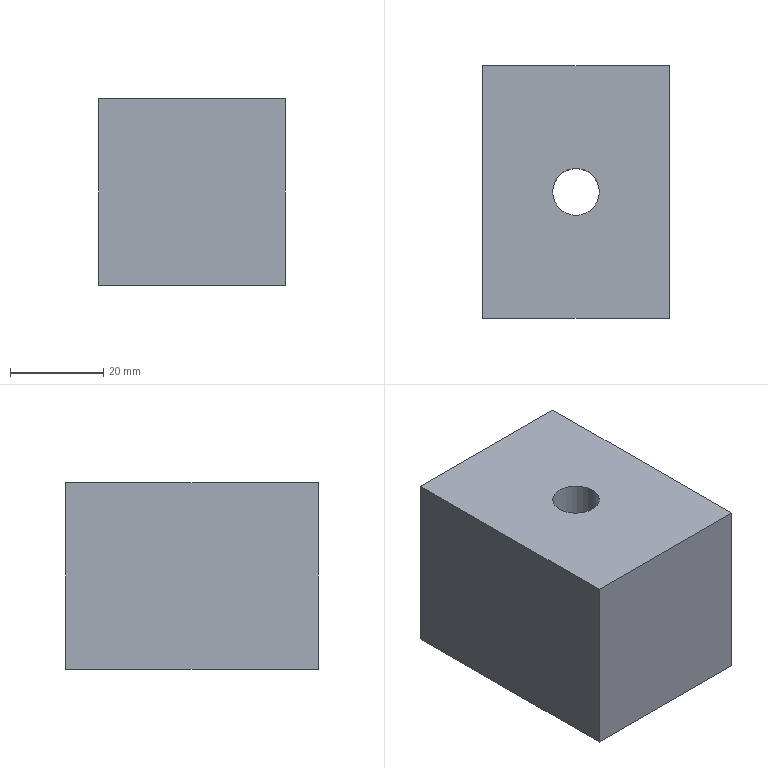Part | STEP file | 1 solid | 8 faces | box 40 x 54 x 40 mm | volume 83258 mm3 | plane 6 | cylinder 2 | commonest cylinder face diameters 10 x2
STEP:
#1=CARTESIAN_POINT('',(0.,0.,0.));
#2=DIRECTION('',(0.,0.,1.));
#3=DIRECTION('',(1.,0.,0.));
#4=AXIS2_PLACEMENT_3D('',#1,#2,#3);
#5=CARTESIAN_POINT('',(5.,0.,0.));
#6=VERTEX_POINT('',#5);
#7=CARTESIAN_POINT('',(5.,0.,40.));
#8=VERTEX_POINT('',#7);
#9=CARTESIAN_POINT('',(5.,0.,40.));
#10=DIRECTION('',(0.,0.,1.));
#11=VECTOR('',#10,1.);
#12=LINE('',#9,#11);
#13=CARTESIAN_POINT('',(0.,0.,40.));
#14=DIRECTION('',(0.,0.,1.));
#15=DIRECTION('',(1.,0.,0.));
#16=AXIS2_PLACEMENT_3D('',#13,#14,#15);
#17=CYLINDRICAL_SURFACE('',#16,5.);
#18=CARTESIAN_POINT('',(6.283,0.));
#19=DIRECTION('',(0.,1.));
#20=VECTOR('',#19,1.);
#21=LINE('',#18,#20);
#22=(GEOMETRIC_REPRESENTATION_CONTEXT(2)PARAMETRIC_REPRESENTATION_CONTEXT()REPRESENTATION_CONTEXT('',''));
#23=DEFINITIONAL_REPRESENTATION('',(#21),#22);
#24=PCURVE('',#17,#23);
#25=CARTESIAN_POINT('',(0.,0.,40.));
#26=DIRECTION('',(0.,0.,1.));
#27=DIRECTION('',(1.,0.,0.));
#28=AXIS2_PLACEMENT_3D('',#25,#26,#27);
#29=CYLINDRICAL_SURFACE('',#28,5.);
#30=CARTESIAN_POINT('',(0.,0.));
#31=DIRECTION('',(0.,1.));
#32=VECTOR('',#31,1.);
#33=LINE('',#30,#32);
#34=(GEOMETRIC_REPRESENTATION_CONTEXT(2)PARAMETRIC_REPRESENTATION_CONTEXT()REPRESENTATION_CONTEXT('',''));
#35=DEFINITIONAL_REPRESENTATION('',(#33),#34);
#36=PCURVE('',#29,#35);
#37=SURFACE_CURVE('',#12,(#24,#36),.PCURVE_S1.);
#38=EDGE_CURVE('',#6,#8,#37,.T.);
#39=ORIENTED_EDGE('',*,*,#38,.T.);
#40=CARTESIAN_POINT('',(-5.,0.,40.));
#41=VERTEX_POINT('',#40);
#42=CARTESIAN_POINT('',(0.,0.,40.));
#43=DIRECTION('',(0.,0.,-1.));
#44=DIRECTION('',(1.,0.,0.));
#45=AXIS2_PLACEMENT_3D('',#42,#43,#44);
#46=CIRCLE('',#45,5.);
#47=CARTESIAN_POINT('',(6.283,0.));
#48=DIRECTION('',(-1.,0.));
#49=VECTOR('',#48,1.);
#50=LINE('',#47,#49);
#51=(GEOMETRIC_REPRESENTATION_CONTEXT(2)PARAMETRIC_REPRESENTATION_CONTEXT()REPRESENTATION_CONTEXT('',''));
#52=DEFINITIONAL_REPRESENTATION('',(#50),#51);
#53=PCURVE('',#17,#52);
#54=CARTESIAN_POINT('',(0.,0.,40.));
#55=DIRECTION('',(0.,0.,1.));
#56=DIRECTION('',(1.,0.,0.));
#57=AXIS2_PLACEMENT_3D('',#54,#55,#56);
#58=PLANE('',#57);
#59=CARTESIAN_POINT('',(5.,0.));
#60=CARTESIAN_POINT('',(5.,-8.66));
#61=CARTESIAN_POINT('',(-2.5,-4.33));
#62=CARTESIAN_POINT('',(-10.,0.));
#63=CARTESIAN_POINT('',(-2.5,4.33));
#64=CARTESIAN_POINT('',(5.,8.66));
#65=CARTESIAN_POINT('',(5.,0.));
#66=(BOUNDED_CURVE()B_SPLINE_CURVE(2,(#59,#60,#61,#62,#63,#64,#65),.UNSPECIFIED.,.T.,.F.)B_SPLINE_CURVE_WITH_KNOTS((1,2,2,2,2,1),(-2.094,0.,2.094,4.189,6.283,8.378),.UNSPECIFIED.)CURVE()GEOMETRIC_REPRESENTATION_ITEM()RATIONAL_B_SPLINE_CURVE((1.,0.5,1.,0.5,1.,0.5,1.))REPRESENTATION_ITEM(''));
#67=(GEOMETRIC_REPRESENTATION_CONTEXT(2)PARAMETRIC_REPRESENTATION_CONTEXT()REPRESENTATION_CONTEXT('',''));
#68=DEFINITIONAL_REPRESENTATION('',(#66),#67);
#69=PCURVE('',#58,#68);
#70=SURFACE_CURVE('',#46,(#53,#69),.PCURVE_S1.);
#71=EDGE_CURVE('',#8,#41,#70,.T.);
#72=ORIENTED_EDGE('',*,*,#71,.T.);
#73=CARTESIAN_POINT('',(-5.,0.,0.));
#74=VERTEX_POINT('',#73);
#75=CARTESIAN_POINT('',(-5.,0.,40.));
#76=DIRECTION('',(0.,0.,1.));
#77=VECTOR('',#76,1.);
#78=LINE('',#75,#77);
#79=CARTESIAN_POINT('',(3.142,0.));
#80=DIRECTION('',(0.,1.));
#81=VECTOR('',#80,1.);
#82=LINE('',#79,#81);
#83=(GEOMETRIC_REPRESENTATION_CONTEXT(2)PARAMETRIC_REPRESENTATION_CONTEXT()REPRESENTATION_CONTEXT('',''));
#84=DEFINITIONAL_REPRESENTATION('',(#82),#83);
#85=PCURVE('',#17,#84);
#86=CARTESIAN_POINT('',(3.142,0.));
#87=DIRECTION('',(0.,1.));
#88=VECTOR('',#87,1.);
#89=LINE('',#86,#88);
#90=(GEOMETRIC_REPRESENTATION_CONTEXT(2)PARAMETRIC_REPRESENTATION_CONTEXT()REPRESENTATION_CONTEXT('',''));
#91=DEFINITIONAL_REPRESENTATION('',(#89),#90);
#92=PCURVE('',#29,#91);
#93=SURFACE_CURVE('',#78,(#85,#92),.PCURVE_S1.);
#94=EDGE_CURVE('',#74,#41,#93,.T.);
#95=ORIENTED_EDGE('',*,*,#94,.F.);
#96=CARTESIAN_POINT('',(0.,0.,0.));
#97=DIRECTION('',(0.,0.,-1.));
#98=DIRECTION('',(1.,0.,0.));
#99=AXIS2_PLACEMENT_3D('',#96,#97,#98);
#100=CIRCLE('',#99,5.);
#101=CARTESIAN_POINT('',(6.283,-40.));
#102=DIRECTION('',(-1.,0.));
#103=VECTOR('',#102,1.);
#104=LINE('',#101,#103);
#105=(GEOMETRIC_REPRESENTATION_CONTEXT(2)PARAMETRIC_REPRESENTATION_CONTEXT()REPRESENTATION_CONTEXT('',''));
#106=DEFINITIONAL_REPRESENTATION('',(#104),#105);
#107=PCURVE('',#17,#106);
#108=CARTESIAN_POINT('',(0.,0.,0.));
#109=DIRECTION('',(0.,0.,1.));
#110=DIRECTION('',(1.,0.,0.));
#111=AXIS2_PLACEMENT_3D('',#108,#109,#110);
#112=PLANE('',#111);
#113=CARTESIAN_POINT('',(5.,0.));
#114=CARTESIAN_POINT('',(5.,-8.66));
#115=CARTESIAN_POINT('',(-2.5,-4.33));
#116=CARTESIAN_POINT('',(-10.,0.));
#117=CARTESIAN_POINT('',(-2.5,4.33));
#118=CARTESIAN_POINT('',(5.,8.66));
#119=CARTESIAN_POINT('',(5.,0.));
#120=(BOUNDED_CURVE()B_SPLINE_CURVE(2,(#113,#114,#115,#116,#117,#118,#119),.UNSPECIFIED.,.T.,.F.)B_SPLINE_CURVE_WITH_KNOTS((1,2,2,2,2,1),(-2.094,0.,2.094,4.189,6.283,8.378),.UNSPECIFIED.)CURVE()GEOMETRIC_REPRESENTATION_ITEM()RATIONAL_B_SPLINE_CURVE((1.,0.5,1.,0.5,1.,0.5,1.))REPRESENTATION_ITEM(''));
#121=(GEOMETRIC_REPRESENTATION_CONTEXT(2)PARAMETRIC_REPRESENTATION_CONTEXT()REPRESENTATION_CONTEXT('',''));
#122=DEFINITIONAL_REPRESENTATION('',(#120),#121);
#123=PCURVE('',#112,#122);
#124=SURFACE_CURVE('',#100,(#107,#123),.PCURVE_S1.);
#125=EDGE_CURVE('',#6,#74,#124,.T.);
#126=ORIENTED_EDGE('',*,*,#125,.F.);
#127=EDGE_LOOP('',(#39,#72,#95,#126));
#128=FACE_BOUND('',#127,.F.);
#129=ADVANCED_FACE('',(#128),#17,.F.);
#130=CARTESIAN_POINT('',(20.,27.,40.));
#131=VERTEX_POINT('',#130);
#132=CARTESIAN_POINT('',(20.,27.,0.));
#133=VERTEX_POINT('',#132);
#134=CARTESIAN_POINT('',(20.,27.,40.));
#135=DIRECTION('',(0.,0.,-1.));
#136=VECTOR('',#135,1.);
#137=LINE('',#134,#136);
#138=CARTESIAN_POINT('',(20.,27.,40.));
#139=DIRECTION('',(-1.,0.,0.));
#140=DIRECTION('',(0.,-1.,0.));
#141=AXIS2_PLACEMENT_3D('',#138,#139,#140);
#142=PLANE('',#141);
#143=CARTESIAN_POINT('',(0.,0.));
#144=DIRECTION('',(0.,-1.));
#145=VECTOR('',#144,1.);
#146=LINE('',#143,#145);
#147=(GEOMETRIC_REPRESENTATION_CONTEXT(2)PARAMETRIC_REPRESENTATION_CONTEXT()REPRESENTATION_CONTEXT('',''));
#148=DEFINITIONAL_REPRESENTATION('',(#146),#147);
#149=PCURVE('',#142,#148);
#150=CARTESIAN_POINT('',(-20.,27.,40.));
#151=DIRECTION('',(0.,-1.,0.));
#152=DIRECTION('',(0.,0.,-1.));
#153=AXIS2_PLACEMENT_3D('',#150,#151,#152);
#154=PLANE('',#153);
#155=CARTESIAN_POINT('',(0.,40.));
#156=DIRECTION('',(1.,0.));
#157=VECTOR('',#156,1.);
#158=LINE('',#155,#157);
#159=(GEOMETRIC_REPRESENTATION_CONTEXT(2)PARAMETRIC_REPRESENTATION_CONTEXT()REPRESENTATION_CONTEXT('',''));
#160=DEFINITIONAL_REPRESENTATION('',(#158),#159);
#161=PCURVE('',#154,#160);
#162=SURFACE_CURVE('',#137,(#149,#161),.PCURVE_S1.);
#163=EDGE_CURVE('',#131,#133,#162,.T.);
#164=ORIENTED_EDGE('',*,*,#163,.F.);
#165=CARTESIAN_POINT('',(20.,-27.,40.));
#166=VERTEX_POINT('',#165);
#167=CARTESIAN_POINT('',(20.,27.,40.));
#168=DIRECTION('',(0.,1.,0.));
#169=VECTOR('',#168,1.);
#170=LINE('',#167,#169);
#171=CARTESIAN_POINT('',(0.,0.));
#172=DIRECTION('',(-1.,0.));
#173=VECTOR('',#172,1.);
#174=LINE('',#171,#173);
#175=(GEOMETRIC_REPRESENTATION_CONTEXT(2)PARAMETRIC_REPRESENTATION_CONTEXT()REPRESENTATION_CONTEXT('',''));
#176=DEFINITIONAL_REPRESENTATION('',(#174),#175);
#177=PCURVE('',#142,#176);
#178=CARTESIAN_POINT('',(20.,27.));
#179=DIRECTION('',(0.,1.));
#180=VECTOR('',#179,1.);
#181=LINE('',#178,#180);
#182=(GEOMETRIC_REPRESENTATION_CONTEXT(2)PARAMETRIC_REPRESENTATION_CONTEXT()REPRESENTATION_CONTEXT('',''));
#183=DEFINITIONAL_REPRESENTATION('',(#181),#182);
#184=PCURVE('',#58,#183);
#185=SURFACE_CURVE('',#170,(#177,#184),.PCURVE_S1.);
#186=EDGE_CURVE('',#166,#131,#185,.T.);
#187=ORIENTED_EDGE('',*,*,#186,.F.);
#188=CARTESIAN_POINT('',(20.,-27.,0.));
#189=VERTEX_POINT('',#188);
#190=CARTESIAN_POINT('',(20.,-27.,40.));
#191=DIRECTION('',(0.,0.,1.));
#192=VECTOR('',#191,1.);
#193=LINE('',#190,#192);
#194=CARTESIAN_POINT('',(54.,0.));
#195=DIRECTION('',(0.,1.));
#196=VECTOR('',#195,1.);
#197=LINE('',#194,#196);
#198=(GEOMETRIC_REPRESENTATION_CONTEXT(2)PARAMETRIC_REPRESENTATION_CONTEXT()REPRESENTATION_CONTEXT('',''));
#199=DEFINITIONAL_REPRESENTATION('',(#197),#198);
#200=PCURVE('',#142,#199);
#201=CARTESIAN_POINT('',(-20.,-27.,40.));
#202=DIRECTION('',(0.,1.,0.));
#203=DIRECTION('',(0.,0.,1.));
#204=AXIS2_PLACEMENT_3D('',#201,#202,#203);
#205=PLANE('',#204);
#206=CARTESIAN_POINT('',(0.,40.));
#207=DIRECTION('',(1.,0.));
#208=VECTOR('',#207,1.);
#209=LINE('',#206,#208);
#210=(GEOMETRIC_REPRESENTATION_CONTEXT(2)PARAMETRIC_REPRESENTATION_CONTEXT()REPRESENTATION_CONTEXT('',''));
#211=DEFINITIONAL_REPRESENTATION('',(#209),#210);
#212=PCURVE('',#205,#211);
#213=SURFACE_CURVE('',#193,(#200,#212),.PCURVE_S1.);
#214=EDGE_CURVE('',#189,#166,#213,.T.);
#215=ORIENTED_EDGE('',*,*,#214,.F.);
#216=CARTESIAN_POINT('',(20.,27.,0.));
#217=DIRECTION('',(0.,-1.,0.));
#218=VECTOR('',#217,1.);
#219=LINE('',#216,#218);
#220=CARTESIAN_POINT('',(0.,-40.));
#221=DIRECTION('',(1.,0.));
#222=VECTOR('',#221,1.);
#223=LINE('',#220,#222);
#224=(GEOMETRIC_REPRESENTATION_CONTEXT(2)PARAMETRIC_REPRESENTATION_CONTEXT()REPRESENTATION_CONTEXT('',''));
#225=DEFINITIONAL_REPRESENTATION('',(#223),#224);
#226=PCURVE('',#142,#225);
#227=CARTESIAN_POINT('',(20.,27.));
#228=DIRECTION('',(0.,-1.));
#229=VECTOR('',#228,1.);
#230=LINE('',#227,#229);
#231=(GEOMETRIC_REPRESENTATION_CONTEXT(2)PARAMETRIC_REPRESENTATION_CONTEXT()REPRESENTATION_CONTEXT('',''));
#232=DEFINITIONAL_REPRESENTATION('',(#230),#231);
#233=PCURVE('',#112,#232);
#234=SURFACE_CURVE('',#219,(#226,#233),.PCURVE_S1.);
#235=EDGE_CURVE('',#133,#189,#234,.T.);
#236=ORIENTED_EDGE('',*,*,#235,.F.);
#237=EDGE_LOOP('',(#164,#187,#215,#236));
#238=FACE_BOUND('',#237,.T.);
#239=ADVANCED_FACE('',(#238),#142,.F.);
#240=ORIENTED_EDGE('',*,*,#125,.F.);
#241=CARTESIAN_POINT('',(0.,0.,0.));
#242=DIRECTION('',(0.,0.,-1.));
#243=DIRECTION('',(1.,0.,0.));
#244=AXIS2_PLACEMENT_3D('',#241,#242,#243);
#245=CIRCLE('',#244,5.);
#246=CARTESIAN_POINT('',(5.,0.));
#247=CARTESIAN_POINT('',(5.,-8.66));
#248=CARTESIAN_POINT('',(-2.5,-4.33));
#249=CARTESIAN_POINT('',(-10.,0.));
#250=CARTESIAN_POINT('',(-2.5,4.33));
#251=CARTESIAN_POINT('',(5.,8.66));
#252=CARTESIAN_POINT('',(5.,0.));
#253=(BOUNDED_CURVE()B_SPLINE_CURVE(2,(#246,#247,#248,#249,#250,#251,#252),.UNSPECIFIED.,.T.,.F.)B_SPLINE_CURVE_WITH_KNOTS((1,2,2,2,2,1),(-2.094,0.,2.094,4.189,6.283,8.378),.UNSPECIFIED.)CURVE()GEOMETRIC_REPRESENTATION_ITEM()RATIONAL_B_SPLINE_CURVE((1.,0.5,1.,0.5,1.,0.5,1.))REPRESENTATION_ITEM(''));
#254=(GEOMETRIC_REPRESENTATION_CONTEXT(2)PARAMETRIC_REPRESENTATION_CONTEXT()REPRESENTATION_CONTEXT('',''));
#255=DEFINITIONAL_REPRESENTATION('',(#253),#254);
#256=PCURVE('',#112,#255);
#257=CARTESIAN_POINT('',(6.283,-40.));
#258=DIRECTION('',(-1.,0.));
#259=VECTOR('',#258,1.);
#260=LINE('',#257,#259);
#261=(GEOMETRIC_REPRESENTATION_CONTEXT(2)PARAMETRIC_REPRESENTATION_CONTEXT()REPRESENTATION_CONTEXT('',''));
#262=DEFINITIONAL_REPRESENTATION('',(#260),#261);
#263=PCURVE('',#29,#262);
#264=SURFACE_CURVE('',#245,(#256,#263),.PCURVE_S1.);
#265=EDGE_CURVE('',#74,#6,#264,.T.);
#266=ORIENTED_EDGE('',*,*,#265,.F.);
#267=EDGE_LOOP('',(#240,#266));
#268=FACE_BOUND('',#267,.T.);
#269=CARTESIAN_POINT('',(-20.,-27.,0.));
#270=VERTEX_POINT('',#269);
#271=CARTESIAN_POINT('',(0.,-27.,0.));
#272=DIRECTION('',(1.,0.,0.));
#273=VECTOR('',#272,1.);
#274=LINE('',#271,#273);
#275=CARTESIAN_POINT('',(0.,-27.));
#276=DIRECTION('',(1.,0.));
#277=VECTOR('',#276,1.);
#278=LINE('',#275,#277);
#279=(GEOMETRIC_REPRESENTATION_CONTEXT(2)PARAMETRIC_REPRESENTATION_CONTEXT()REPRESENTATION_CONTEXT('',''));
#280=DEFINITIONAL_REPRESENTATION('',(#278),#279);
#281=PCURVE('',#112,#280);
#282=CARTESIAN_POINT('',(-40.,20.));
#283=DIRECTION('',(0.,1.));
#284=VECTOR('',#283,1.);
#285=LINE('',#282,#284);
#286=(GEOMETRIC_REPRESENTATION_CONTEXT(2)PARAMETRIC_REPRESENTATION_CONTEXT()REPRESENTATION_CONTEXT('',''));
#287=DEFINITIONAL_REPRESENTATION('',(#285),#286);
#288=PCURVE('',#205,#287);
#289=SURFACE_CURVE('',#274,(#281,#288),.PCURVE_S1.);
#290=EDGE_CURVE('',#270,#189,#289,.T.);
#291=ORIENTED_EDGE('',*,*,#290,.F.);
#292=CARTESIAN_POINT('',(-20.,27.,0.));
#293=VERTEX_POINT('',#292);
#294=CARTESIAN_POINT('',(-20.,0.,0.));
#295=DIRECTION('',(0.,-1.,0.));
#296=VECTOR('',#295,1.);
#297=LINE('',#294,#296);
#298=CARTESIAN_POINT('',(-20.,0.));
#299=DIRECTION('',(0.,-1.));
#300=VECTOR('',#299,1.);
#301=LINE('',#298,#300);
#302=(GEOMETRIC_REPRESENTATION_CONTEXT(2)PARAMETRIC_REPRESENTATION_CONTEXT()REPRESENTATION_CONTEXT('',''));
#303=DEFINITIONAL_REPRESENTATION('',(#301),#302);
#304=PCURVE('',#112,#303);
#305=CARTESIAN_POINT('',(-20.,27.,40.));
#306=DIRECTION('',(1.,0.,0.));
#307=DIRECTION('',(0.,1.,0.));
#308=AXIS2_PLACEMENT_3D('',#305,#306,#307);
#309=PLANE('',#308);
#310=CARTESIAN_POINT('',(-27.,-40.));
#311=DIRECTION('',(-1.,0.));
#312=VECTOR('',#311,1.);
#313=LINE('',#310,#312);
#314=(GEOMETRIC_REPRESENTATION_CONTEXT(2)PARAMETRIC_REPRESENTATION_CONTEXT()REPRESENTATION_CONTEXT('',''));
#315=DEFINITIONAL_REPRESENTATION('',(#313),#314);
#316=PCURVE('',#309,#315);
#317=SURFACE_CURVE('',#297,(#304,#316),.PCURVE_S1.);
#318=EDGE_CURVE('',#293,#270,#317,.T.);
#319=ORIENTED_EDGE('',*,*,#318,.F.);
#320=CARTESIAN_POINT('',(0.,27.,0.));
#321=DIRECTION('',(-1.,0.,0.));
#322=VECTOR('',#321,1.);
#323=LINE('',#320,#322);
#324=CARTESIAN_POINT('',(0.,27.));
#325=DIRECTION('',(-1.,0.));
#326=VECTOR('',#325,1.);
#327=LINE('',#324,#326);
#328=(GEOMETRIC_REPRESENTATION_CONTEXT(2)PARAMETRIC_REPRESENTATION_CONTEXT()REPRESENTATION_CONTEXT('',''));
#329=DEFINITIONAL_REPRESENTATION('',(#327),#328);
#330=PCURVE('',#112,#329);
#331=CARTESIAN_POINT('',(40.,20.));
#332=DIRECTION('',(0.,-1.));
#333=VECTOR('',#332,1.);
#334=LINE('',#331,#333);
#335=(GEOMETRIC_REPRESENTATION_CONTEXT(2)PARAMETRIC_REPRESENTATION_CONTEXT()REPRESENTATION_CONTEXT('',''));
#336=DEFINITIONAL_REPRESENTATION('',(#334),#335);
#337=PCURVE('',#154,#336);
#338=SURFACE_CURVE('',#323,(#330,#337),.PCURVE_S1.);
#339=EDGE_CURVE('',#133,#293,#338,.T.);
#340=ORIENTED_EDGE('',*,*,#339,.F.);
#341=ORIENTED_EDGE('',*,*,#235,.T.);
#342=EDGE_LOOP('',(#291,#319,#340,#341));
#343=FACE_BOUND('',#342,.T.);
#344=ADVANCED_FACE('',(#268,#343),#112,.F.);
#345=CARTESIAN_POINT('',(-20.,27.,40.));
#346=VERTEX_POINT('',#345);
#347=CARTESIAN_POINT('',(-20.,27.,40.));
#348=DIRECTION('',(0.,0.,-1.));
#349=VECTOR('',#348,1.);
#350=LINE('',#347,#349);
#351=CARTESIAN_POINT('',(0.,0.));
#352=DIRECTION('',(1.,0.));
#353=VECTOR('',#352,1.);
#354=LINE('',#351,#353);
#355=(GEOMETRIC_REPRESENTATION_CONTEXT(2)PARAMETRIC_REPRESENTATION_CONTEXT()REPRESENTATION_CONTEXT('',''));
#356=DEFINITIONAL_REPRESENTATION('',(#354),#355);
#357=PCURVE('',#154,#356);
#358=CARTESIAN_POINT('',(0.,0.));
#359=DIRECTION('',(0.,-1.));
#360=VECTOR('',#359,1.);
#361=LINE('',#358,#360);
#362=(GEOMETRIC_REPRESENTATION_CONTEXT(2)PARAMETRIC_REPRESENTATION_CONTEXT()REPRESENTATION_CONTEXT('',''));
#363=DEFINITIONAL_REPRESENTATION('',(#361),#362);
#364=PCURVE('',#309,#363);
#365=SURFACE_CURVE('',#350,(#357,#364),.PCURVE_S1.);
#366=EDGE_CURVE('',#346,#293,#365,.T.);
#367=ORIENTED_EDGE('',*,*,#366,.F.);
#368=CARTESIAN_POINT('',(-20.,27.,40.));
#369=DIRECTION('',(-1.,0.,0.));
#370=VECTOR('',#369,1.);
#371=LINE('',#368,#370);
#372=CARTESIAN_POINT('',(0.,0.));
#373=DIRECTION('',(0.,-1.));
#374=VECTOR('',#373,1.);
#375=LINE('',#372,#374);
#376=(GEOMETRIC_REPRESENTATION_CONTEXT(2)PARAMETRIC_REPRESENTATION_CONTEXT()REPRESENTATION_CONTEXT('',''));
#377=DEFINITIONAL_REPRESENTATION('',(#375),#376);
#378=PCURVE('',#154,#377);
#379=CARTESIAN_POINT('',(-20.,27.));
#380=DIRECTION('',(-1.,0.));
#381=VECTOR('',#380,1.);
#382=LINE('',#379,#381);
#383=(GEOMETRIC_REPRESENTATION_CONTEXT(2)PARAMETRIC_REPRESENTATION_CONTEXT()REPRESENTATION_CONTEXT('',''));
#384=DEFINITIONAL_REPRESENTATION('',(#382),#383);
#385=PCURVE('',#58,#384);
#386=SURFACE_CURVE('',#371,(#378,#385),.PCURVE_S1.);
#387=EDGE_CURVE('',#131,#346,#386,.T.);
#388=ORIENTED_EDGE('',*,*,#387,.F.);
#389=ORIENTED_EDGE('',*,*,#163,.T.);
#390=ORIENTED_EDGE('',*,*,#339,.T.);
#391=EDGE_LOOP('',(#367,#388,#389,#390));
#392=FACE_BOUND('',#391,.T.);
#393=ADVANCED_FACE('',(#392),#154,.F.);
#394=ORIENTED_EDGE('',*,*,#71,.T.);
#395=CARTESIAN_POINT('',(0.,0.,40.));
#396=DIRECTION('',(0.,0.,-1.));
#397=DIRECTION('',(1.,0.,0.));
#398=AXIS2_PLACEMENT_3D('',#395,#396,#397);
#399=CIRCLE('',#398,5.);
#400=CARTESIAN_POINT('',(5.,0.));
#401=CARTESIAN_POINT('',(5.,-8.66));
#402=CARTESIAN_POINT('',(-2.5,-4.33));
#403=CARTESIAN_POINT('',(-10.,0.));
#404=CARTESIAN_POINT('',(-2.5,4.33));
#405=CARTESIAN_POINT('',(5.,8.66));
#406=CARTESIAN_POINT('',(5.,0.));
#407=(BOUNDED_CURVE()B_SPLINE_CURVE(2,(#400,#401,#402,#403,#404,#405,#406),.UNSPECIFIED.,.T.,.F.)B_SPLINE_CURVE_WITH_KNOTS((1,2,2,2,2,1),(-2.094,0.,2.094,4.189,6.283,8.378),.UNSPECIFIED.)CURVE()GEOMETRIC_REPRESENTATION_ITEM()RATIONAL_B_SPLINE_CURVE((1.,0.5,1.,0.5,1.,0.5,1.))REPRESENTATION_ITEM(''));
#408=(GEOMETRIC_REPRESENTATION_CONTEXT(2)PARAMETRIC_REPRESENTATION_CONTEXT()REPRESENTATION_CONTEXT('',''));
#409=DEFINITIONAL_REPRESENTATION('',(#407),#408);
#410=PCURVE('',#58,#409);
#411=CARTESIAN_POINT('',(6.283,0.));
#412=DIRECTION('',(-1.,0.));
#413=VECTOR('',#412,1.);
#414=LINE('',#411,#413);
#415=(GEOMETRIC_REPRESENTATION_CONTEXT(2)PARAMETRIC_REPRESENTATION_CONTEXT()REPRESENTATION_CONTEXT('',''));
#416=DEFINITIONAL_REPRESENTATION('',(#414),#415);
#417=PCURVE('',#29,#416);
#418=SURFACE_CURVE('',#399,(#410,#417),.PCURVE_S1.);
#419=EDGE_CURVE('',#41,#8,#418,.T.);
#420=ORIENTED_EDGE('',*,*,#419,.T.);
#421=EDGE_LOOP('',(#394,#420));
#422=FACE_BOUND('',#421,.T.);
#423=CARTESIAN_POINT('',(-20.,-27.,40.));
#424=VERTEX_POINT('',#423);
#425=CARTESIAN_POINT('',(-20.,0.,40.));
#426=DIRECTION('',(0.,-1.,0.));
#427=VECTOR('',#426,1.);
#428=LINE('',#425,#427);
#429=CARTESIAN_POINT('',(-20.,0.));
#430=DIRECTION('',(0.,-1.));
#431=VECTOR('',#430,1.);
#432=LINE('',#429,#431);
#433=(GEOMETRIC_REPRESENTATION_CONTEXT(2)PARAMETRIC_REPRESENTATION_CONTEXT()REPRESENTATION_CONTEXT('',''));
#434=DEFINITIONAL_REPRESENTATION('',(#432),#433);
#435=PCURVE('',#58,#434);
#436=CARTESIAN_POINT('',(-27.,0.));
#437=DIRECTION('',(-1.,0.));
#438=VECTOR('',#437,1.);
#439=LINE('',#436,#438);
#440=(GEOMETRIC_REPRESENTATION_CONTEXT(2)PARAMETRIC_REPRESENTATION_CONTEXT()REPRESENTATION_CONTEXT('',''));
#441=DEFINITIONAL_REPRESENTATION('',(#439),#440);
#442=PCURVE('',#309,#441);
#443=SURFACE_CURVE('',#428,(#435,#442),.PCURVE_S1.);
#444=EDGE_CURVE('',#346,#424,#443,.T.);
#445=ORIENTED_EDGE('',*,*,#444,.T.);
#446=CARTESIAN_POINT('',(0.,-27.,40.));
#447=DIRECTION('',(1.,0.,0.));
#448=VECTOR('',#447,1.);
#449=LINE('',#446,#448);
#450=CARTESIAN_POINT('',(0.,-27.));
#451=DIRECTION('',(1.,0.));
#452=VECTOR('',#451,1.);
#453=LINE('',#450,#452);
#454=(GEOMETRIC_REPRESENTATION_CONTEXT(2)PARAMETRIC_REPRESENTATION_CONTEXT()REPRESENTATION_CONTEXT('',''));
#455=DEFINITIONAL_REPRESENTATION('',(#453),#454);
#456=PCURVE('',#58,#455);
#457=CARTESIAN_POINT('',(0.,20.));
#458=DIRECTION('',(0.,1.));
#459=VECTOR('',#458,1.);
#460=LINE('',#457,#459);
#461=(GEOMETRIC_REPRESENTATION_CONTEXT(2)PARAMETRIC_REPRESENTATION_CONTEXT()REPRESENTATION_CONTEXT('',''));
#462=DEFINITIONAL_REPRESENTATION('',(#460),#461);
#463=PCURVE('',#205,#462);
#464=SURFACE_CURVE('',#449,(#456,#463),.PCURVE_S1.);
#465=EDGE_CURVE('',#424,#166,#464,.T.);
#466=ORIENTED_EDGE('',*,*,#465,.T.);
#467=ORIENTED_EDGE('',*,*,#186,.T.);
#468=ORIENTED_EDGE('',*,*,#387,.T.);
#469=EDGE_LOOP('',(#445,#466,#467,#468));
#470=FACE_BOUND('',#469,.T.);
#471=ADVANCED_FACE('',(#422,#470),#58,.T.);
#472=ORIENTED_EDGE('',*,*,#214,.T.);
#473=ORIENTED_EDGE('',*,*,#465,.F.);
#474=CARTESIAN_POINT('',(-20.,-27.,40.));
#475=DIRECTION('',(0.,0.,1.));
#476=VECTOR('',#475,1.);
#477=LINE('',#474,#476);
#478=CARTESIAN_POINT('',(0.,0.));
#479=DIRECTION('',(1.,0.));
#480=VECTOR('',#479,1.);
#481=LINE('',#478,#480);
#482=(GEOMETRIC_REPRESENTATION_CONTEXT(2)PARAMETRIC_REPRESENTATION_CONTEXT()REPRESENTATION_CONTEXT('',''));
#483=DEFINITIONAL_REPRESENTATION('',(#481),#482);
#484=PCURVE('',#205,#483);
#485=CARTESIAN_POINT('',(-54.,0.));
#486=DIRECTION('',(0.,1.));
#487=VECTOR('',#486,1.);
#488=LINE('',#485,#487);
#489=(GEOMETRIC_REPRESENTATION_CONTEXT(2)PARAMETRIC_REPRESENTATION_CONTEXT()REPRESENTATION_CONTEXT('',''));
#490=DEFINITIONAL_REPRESENTATION('',(#488),#489);
#491=PCURVE('',#309,#490);
#492=SURFACE_CURVE('',#477,(#484,#491),.PCURVE_S1.);
#493=EDGE_CURVE('',#270,#424,#492,.T.);
#494=ORIENTED_EDGE('',*,*,#493,.F.);
#495=ORIENTED_EDGE('',*,*,#290,.T.);
#496=EDGE_LOOP('',(#472,#473,#494,#495));
#497=FACE_BOUND('',#496,.T.);
#498=ADVANCED_FACE('',(#497),#205,.F.);
#499=ORIENTED_EDGE('',*,*,#419,.T.);
#500=ORIENTED_EDGE('',*,*,#38,.F.);
#501=ORIENTED_EDGE('',*,*,#265,.F.);
#502=ORIENTED_EDGE('',*,*,#94,.T.);
#503=EDGE_LOOP('',(#499,#500,#501,#502));
#504=FACE_BOUND('',#503,.F.);
#505=ADVANCED_FACE('',(#504),#29,.F.);
#506=ORIENTED_EDGE('',*,*,#493,.T.);
#507=ORIENTED_EDGE('',*,*,#444,.F.);
#508=ORIENTED_EDGE('',*,*,#366,.T.);
#509=ORIENTED_EDGE('',*,*,#318,.T.);
#510=EDGE_LOOP('',(#506,#507,#508,#509));
#511=FACE_BOUND('',#510,.T.);
#512=ADVANCED_FACE('',(#511),#309,.F.);
#513=CLOSED_SHELL('',(#129,#239,#344,#393,#471,#498,#505,#512));
#514=MANIFOLD_SOLID_BREP('',#513);
#515=(LENGTH_UNIT()NAMED_UNIT(*)SI_UNIT(.MILLI.,.METRE.));
#516=UNCERTAINTY_MEASURE_WITH_UNIT(LENGTH_MEASURE(0.0000001),#515,'','');
#517=(NAMED_UNIT(*)PLANE_ANGLE_UNIT()SI_UNIT($,.RADIAN.));
#518=(NAMED_UNIT(*)SI_UNIT($,.STERADIAN.)SOLID_ANGLE_UNIT());
#519=(GEOMETRIC_REPRESENTATION_CONTEXT(3)GLOBAL_UNCERTAINTY_ASSIGNED_CONTEXT((#516))GLOBAL_UNIT_ASSIGNED_CONTEXT((#515,#517,#518))REPRESENTATION_CONTEXT('',''));
#520=ADVANCED_BREP_SHAPE_REPRESENTATION('',(#4,#514),#519);